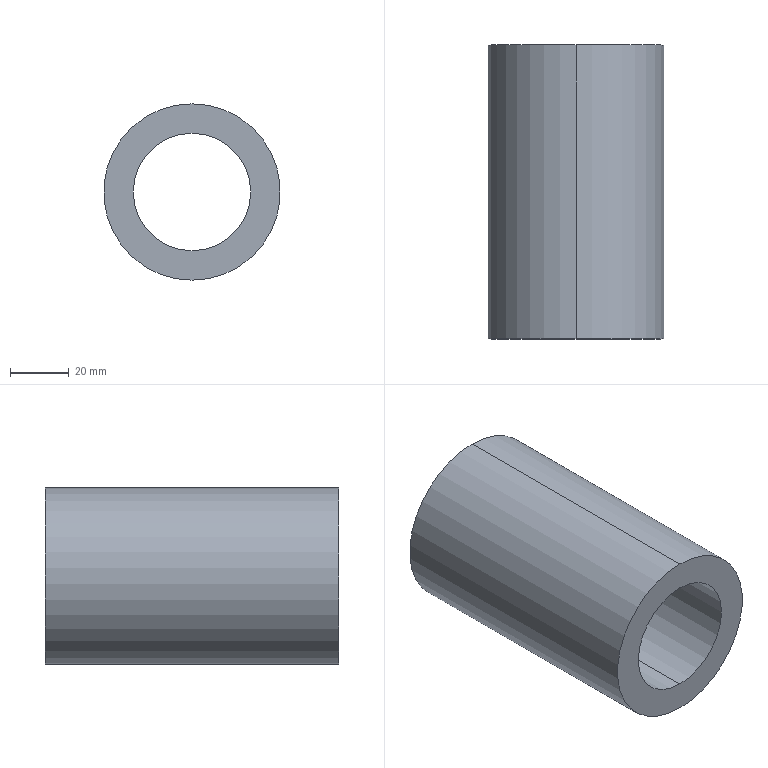Part | SolidWorks | features BaseBody 1 | 1 solid | 6 faces | box 60 x 100 x 60 mm | volume 157080 mm3 | cylinder 4 | plane 2 | commonest cylinder face diameters 40 x2 60 x2
STEP:
#1=CARTESIAN_POINT('',(0.,0.,30.));
#2=VERTEX_POINT('',#1);
#3=CARTESIAN_POINT('',(0.,0.,-30.));
#4=VERTEX_POINT('',#3);
#5=CARTESIAN_POINT('',(0.,0.,0.));
#6=DIRECTION('',(0.,1.,0.));
#7=DIRECTION('',(0.,0.,1.));
#8=AXIS2_PLACEMENT_3D('',#5,#6,#7);
#9=CIRCLE('',#8,30.);
#10=EDGE_CURVE('',#2,#4,#9,.T.);
#11=ORIENTED_EDGE('',*,*,#10,.T.);
#12=CARTESIAN_POINT('',(0.,100.,-30.));
#13=VERTEX_POINT('',#12);
#14=CARTESIAN_POINT('',(0.,0.,-30.));
#15=DIRECTION('',(0.,1.,0.));
#16=VECTOR('',#15,1000.);
#17=LINE('',#14,#16);
#18=EDGE_CURVE('',#4,#13,#17,.T.);
#19=ORIENTED_EDGE('',*,*,#18,.T.);
#20=CARTESIAN_POINT('',(0.,100.,30.));
#21=VERTEX_POINT('',#20);
#22=CARTESIAN_POINT('',(0.,100.,0.));
#23=DIRECTION('',(0.,-1.,0.));
#24=DIRECTION('',(0.,0.,1.));
#25=AXIS2_PLACEMENT_3D('',#22,#23,#24);
#26=CIRCLE('',#25,30.);
#27=EDGE_CURVE('',#13,#21,#26,.T.);
#28=ORIENTED_EDGE('',*,*,#27,.T.);
#29=CARTESIAN_POINT('',(0.,0.,30.));
#30=DIRECTION('',(0.,1.,0.));
#31=VECTOR('',#30,1000.);
#32=LINE('',#29,#31);
#33=EDGE_CURVE('',#2,#21,#32,.T.);
#34=ORIENTED_EDGE('',*,*,#33,.F.);
#35=EDGE_LOOP('',(#11,#19,#28,#34));
#36=FACE_OUTER_BOUND('',#35,.T.);
#37=CARTESIAN_POINT('',(0.,0.,0.));
#38=DIRECTION('',(0.,1.,0.));
#39=DIRECTION('',(0.,0.,1.));
#40=AXIS2_PLACEMENT_3D('',#37,#38,#39);
#41=CYLINDRICAL_SURFACE('',#40,30.);
#42=ADVANCED_FACE('',(#36),#41,.T.);
#43=CARTESIAN_POINT('',(0.,0.,20.));
#44=VERTEX_POINT('',#43);
#45=CARTESIAN_POINT('',(0.,0.,-20.));
#46=VERTEX_POINT('',#45);
#47=CARTESIAN_POINT('',(0.,0.,0.));
#48=DIRECTION('',(0.,-1.,0.));
#49=DIRECTION('',(0.,0.,1.));
#50=AXIS2_PLACEMENT_3D('',#47,#48,#49);
#51=CIRCLE('',#50,20.);
#52=EDGE_CURVE('',#44,#46,#51,.T.);
#53=ORIENTED_EDGE('',*,*,#52,.T.);
#54=CARTESIAN_POINT('',(0.,100.,-20.));
#55=VERTEX_POINT('',#54);
#56=CARTESIAN_POINT('',(0.,0.,-20.));
#57=DIRECTION('',(0.,1.,0.));
#58=VECTOR('',#57,1000.);
#59=LINE('',#56,#58);
#60=EDGE_CURVE('',#46,#55,#59,.T.);
#61=ORIENTED_EDGE('',*,*,#60,.T.);
#62=CARTESIAN_POINT('',(0.,100.,20.));
#63=VERTEX_POINT('',#62);
#64=CARTESIAN_POINT('',(0.,100.,0.));
#65=DIRECTION('',(0.,-1.,0.));
#66=DIRECTION('',(0.,0.,1.));
#67=AXIS2_PLACEMENT_3D('',#64,#65,#66);
#68=CIRCLE('',#67,20.);
#69=EDGE_CURVE('',#63,#55,#68,.T.);
#70=ORIENTED_EDGE('',*,*,#69,.F.);
#71=CARTESIAN_POINT('',(0.,0.,20.));
#72=DIRECTION('',(0.,1.,0.));
#73=VECTOR('',#72,1000.);
#74=LINE('',#71,#73);
#75=EDGE_CURVE('',#44,#63,#74,.T.);
#76=ORIENTED_EDGE('',*,*,#75,.F.);
#77=EDGE_LOOP('',(#53,#61,#70,#76));
#78=FACE_OUTER_BOUND('',#77,.T.);
#79=CARTESIAN_POINT('',(0.,0.,0.));
#80=DIRECTION('',(0.,1.,0.));
#81=DIRECTION('',(0.,0.,1.));
#82=AXIS2_PLACEMENT_3D('',#79,#80,#81);
#83=CYLINDRICAL_SURFACE('',#82,20.);
#84=ADVANCED_FACE('',(#78),#83,.F.);
#85=ORIENTED_EDGE('',*,*,#18,.F.);
#86=CARTESIAN_POINT('',(0.,0.,0.));
#87=DIRECTION('',(0.,1.,0.));
#88=DIRECTION('',(0.,0.,1.));
#89=AXIS2_PLACEMENT_3D('',#86,#87,#88);
#90=CIRCLE('',#89,30.);
#91=EDGE_CURVE('',#4,#2,#90,.T.);
#92=ORIENTED_EDGE('',*,*,#91,.T.);
#93=ORIENTED_EDGE('',*,*,#33,.T.);
#94=CARTESIAN_POINT('',(0.,100.,0.));
#95=DIRECTION('',(0.,-1.,0.));
#96=DIRECTION('',(0.,0.,1.));
#97=AXIS2_PLACEMENT_3D('',#94,#95,#96);
#98=CIRCLE('',#97,30.);
#99=EDGE_CURVE('',#21,#13,#98,.T.);
#100=ORIENTED_EDGE('',*,*,#99,.T.);
#101=EDGE_LOOP('',(#85,#92,#93,#100));
#102=FACE_OUTER_BOUND('',#101,.T.);
#103=CARTESIAN_POINT('',(0.,0.,0.));
#104=DIRECTION('',(0.,1.,0.));
#105=DIRECTION('',(0.,0.,1.));
#106=AXIS2_PLACEMENT_3D('',#103,#104,#105);
#107=CYLINDRICAL_SURFACE('',#106,30.);
#108=ADVANCED_FACE('',(#102),#107,.T.);
#109=ORIENTED_EDGE('',*,*,#52,.F.);
#110=CARTESIAN_POINT('',(0.,0.,0.));
#111=DIRECTION('',(0.,-1.,0.));
#112=DIRECTION('',(0.,0.,1.));
#113=AXIS2_PLACEMENT_3D('',#110,#111,#112);
#114=CIRCLE('',#113,20.);
#115=EDGE_CURVE('',#46,#44,#114,.T.);
#116=ORIENTED_EDGE('',*,*,#115,.F.);
#117=EDGE_LOOP('',(#109,#116));
#118=FACE_BOUND('',#117,.T.);
#119=ORIENTED_EDGE('',*,*,#10,.F.);
#120=ORIENTED_EDGE('',*,*,#91,.F.);
#121=EDGE_LOOP('',(#119,#120));
#122=FACE_OUTER_BOUND('',#121,.T.);
#123=CARTESIAN_POINT('',(0.,0.,0.));
#124=DIRECTION('',(0.,1.,0.));
#125=DIRECTION('',(0.,0.,1.));
#126=AXIS2_PLACEMENT_3D('',#123,#124,#125);
#127=PLANE('',#126);
#128=ADVANCED_FACE('',(#118,#122),#127,.F.);
#129=ORIENTED_EDGE('',*,*,#69,.T.);
#130=CARTESIAN_POINT('',(0.,100.,0.));
#131=DIRECTION('',(0.,-1.,0.));
#132=DIRECTION('',(0.,0.,1.));
#133=AXIS2_PLACEMENT_3D('',#130,#131,#132);
#134=CIRCLE('',#133,20.);
#135=EDGE_CURVE('',#55,#63,#134,.T.);
#136=ORIENTED_EDGE('',*,*,#135,.T.);
#137=EDGE_LOOP('',(#129,#136));
#138=FACE_BOUND('',#137,.T.);
#139=ORIENTED_EDGE('',*,*,#99,.F.);
#140=ORIENTED_EDGE('',*,*,#27,.F.);
#141=EDGE_LOOP('',(#139,#140));
#142=FACE_OUTER_BOUND('',#141,.T.);
#143=CARTESIAN_POINT('',(0.,100.,0.));
#144=DIRECTION('',(0.,1.,0.));
#145=DIRECTION('',(0.,0.,1.));
#146=AXIS2_PLACEMENT_3D('',#143,#144,#145);
#147=PLANE('',#146);
#148=ADVANCED_FACE('',(#138,#142),#147,.T.);
#149=ORIENTED_EDGE('',*,*,#60,.F.);
#150=ORIENTED_EDGE('',*,*,#115,.T.);
#151=ORIENTED_EDGE('',*,*,#75,.T.);
#152=ORIENTED_EDGE('',*,*,#135,.F.);
#153=EDGE_LOOP('',(#149,#150,#151,#152));
#154=FACE_OUTER_BOUND('',#153,.T.);
#155=CARTESIAN_POINT('',(0.,0.,0.));
#156=DIRECTION('',(0.,1.,0.));
#157=DIRECTION('',(0.,0.,1.));
#158=AXIS2_PLACEMENT_3D('',#155,#156,#157);
#159=CYLINDRICAL_SURFACE('',#158,20.);
#160=ADVANCED_FACE('',(#154),#159,.F.);
#161=CLOSED_SHELL('',(#42,#84,#108,#128,#148,#160));
#162=MANIFOLD_SOLID_BREP('',#161);
#163=CARTESIAN_POINT('',(0.,0.,0.));
#164=DIRECTION('',(0.,0.,1.));
#165=DIRECTION('',(1.,0.,0.));
#166=AXIS2_PLACEMENT_3D('',#163,#164,#165);
#167=(LENGTH_UNIT()NAMED_UNIT(*)SI_UNIT(.MILLI.,.METRE.));
#168=UNCERTAINTY_MEASURE_WITH_UNIT(LENGTH_MEASURE(0.00001),#167,'','');
#169=(NAMED_UNIT(*)PLANE_ANGLE_UNIT()SI_UNIT($,.RADIAN.));
#170=(NAMED_UNIT(*)SI_UNIT($,.STERADIAN.)SOLID_ANGLE_UNIT());
#171=(GEOMETRIC_REPRESENTATION_CONTEXT(3)GLOBAL_UNCERTAINTY_ASSIGNED_CONTEXT((#168))GLOBAL_UNIT_ASSIGNED_CONTEXT((#167,#169,#170))REPRESENTATION_CONTEXT('',''));
#172=ADVANCED_BREP_SHAPE_REPRESENTATION('',(#162,#166),#171);